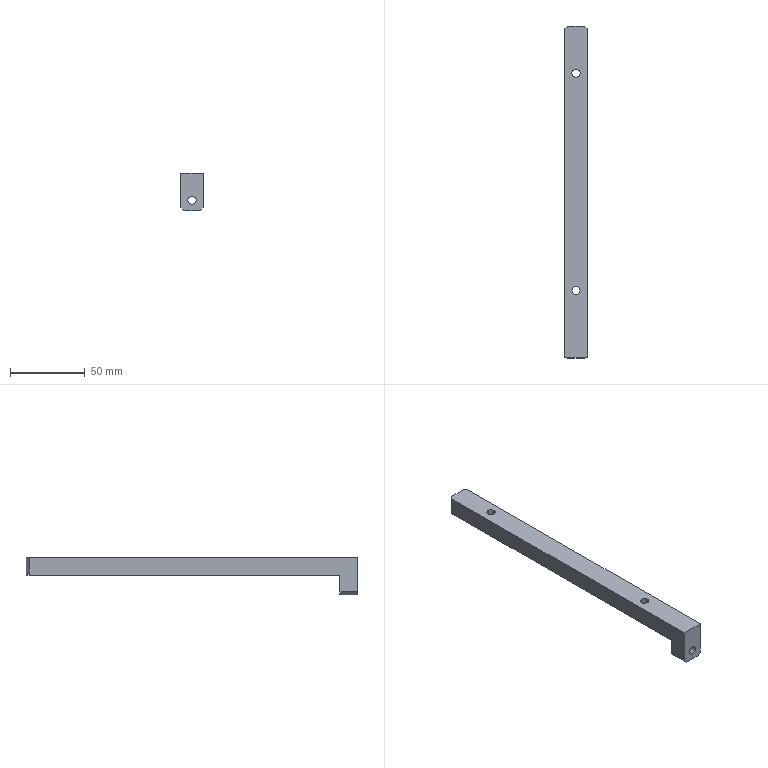Part | SolidWorks | features HoleWzd 2, Chamfer 1, Extrusion 1 | 1 solid | 24 faces | box 15 x 221.5 x 25 mm | volume 40634 mm3 | plane 14 | cylinder 10 | commonest cylinder face diameters 5.5 x6 10 x4
STEP:
#1=CARTESIAN_POINT('',(7.5,12.,-15.25));
#2=VERTEX_POINT('',#1);
#3=CARTESIAN_POINT('',(7.5,12.,-20.75));
#4=VERTEX_POINT('',#3);
#5=CARTESIAN_POINT('',(7.5,12.,-18.));
#6=DIRECTION('',(0.,-1.,0.));
#7=DIRECTION('',(0.,0.,-1.));
#8=AXIS2_PLACEMENT_3D('',#5,#6,#7);
#9=CIRCLE('',#8,2.75);
#10=EDGE_CURVE('',#2,#4,#9,.T.);
#11=ORIENTED_EDGE('',*,*,#10,.F.);
#12=CARTESIAN_POINT('',(7.5,0.,-15.25));
#13=VERTEX_POINT('',#12);
#14=CARTESIAN_POINT('',(7.5,0.,-15.25));
#15=DIRECTION('',(0.,-1.,0.));
#16=VECTOR('',#15,1000.);
#17=LINE('',#14,#16);
#18=EDGE_CURVE('',#2,#13,#17,.T.);
#19=ORIENTED_EDGE('',*,*,#18,.T.);
#20=CARTESIAN_POINT('',(7.5,0.,-20.75));
#21=VERTEX_POINT('',#20);
#22=CARTESIAN_POINT('',(7.5,0.,-18.));
#23=DIRECTION('',(0.,-1.,0.));
#24=DIRECTION('',(0.,0.,-1.));
#25=AXIS2_PLACEMENT_3D('',#22,#23,#24);
#26=CIRCLE('',#25,2.75);
#27=EDGE_CURVE('',#13,#21,#26,.T.);
#28=ORIENTED_EDGE('',*,*,#27,.T.);
#29=CARTESIAN_POINT('',(7.5,0.,-20.75));
#30=DIRECTION('',(0.,-1.,0.));
#31=VECTOR('',#30,1000.);
#32=LINE('',#29,#31);
#33=EDGE_CURVE('',#4,#21,#32,.T.);
#34=ORIENTED_EDGE('',*,*,#33,.F.);
#35=EDGE_LOOP('',(#11,#19,#28,#34));
#36=FACE_OUTER_BOUND('',#35,.T.);
#37=CARTESIAN_POINT('',(7.5,0.,-18.));
#38=DIRECTION('',(0.,-1.,0.));
#39=DIRECTION('',(0.,0.,-1.));
#40=AXIS2_PLACEMENT_3D('',#37,#38,#39);
#41=CYLINDRICAL_SURFACE('',#40,2.75);
#42=ADVANCED_FACE('',(#36),#41,.F.);
#43=CARTESIAN_POINT('',(7.5,185.,-6.3));
#44=VERTEX_POINT('',#43);
#45=CARTESIAN_POINT('',(7.5,195.,-6.3));
#46=VERTEX_POINT('',#45);
#47=CARTESIAN_POINT('',(7.5,190.,-6.3));
#48=DIRECTION('',(0.,0.,-1.));
#49=DIRECTION('',(0.,1.,0.));
#50=AXIS2_PLACEMENT_3D('',#47,#48,#49);
#51=CIRCLE('',#50,5.);
#52=EDGE_CURVE('',#44,#46,#51,.T.);
#53=ORIENTED_EDGE('',*,*,#52,.F.);
#54=CARTESIAN_POINT('',(7.5,185.,-12.));
#55=VERTEX_POINT('',#54);
#56=CARTESIAN_POINT('',(7.5,185.,-12.));
#57=DIRECTION('',(0.,0.,-1.));
#58=VECTOR('',#57,1000.);
#59=LINE('',#56,#58);
#60=EDGE_CURVE('',#44,#55,#59,.T.);
#61=ORIENTED_EDGE('',*,*,#60,.T.);
#62=CARTESIAN_POINT('',(7.5,195.,-12.));
#63=VERTEX_POINT('',#62);
#64=CARTESIAN_POINT('',(7.5,190.,-12.));
#65=DIRECTION('',(0.,0.,-1.));
#66=DIRECTION('',(0.,1.,0.));
#67=AXIS2_PLACEMENT_3D('',#64,#65,#66);
#68=CIRCLE('',#67,5.);
#69=EDGE_CURVE('',#55,#63,#68,.T.);
#70=ORIENTED_EDGE('',*,*,#69,.T.);
#71=CARTESIAN_POINT('',(7.5,195.,-12.));
#72=DIRECTION('',(0.,0.,-1.));
#73=VECTOR('',#72,1000.);
#74=LINE('',#71,#73);
#75=EDGE_CURVE('',#46,#63,#74,.T.);
#76=ORIENTED_EDGE('',*,*,#75,.F.);
#77=EDGE_LOOP('',(#53,#61,#70,#76));
#78=FACE_OUTER_BOUND('',#77,.T.);
#79=CARTESIAN_POINT('',(7.5,190.,-12.));
#80=DIRECTION('',(0.,0.,-1.));
#81=DIRECTION('',(0.,1.,0.));
#82=AXIS2_PLACEMENT_3D('',#79,#80,#81);
#83=CYLINDRICAL_SURFACE('',#82,5.);
#84=ADVANCED_FACE('',(#78),#83,.F.);
#85=CARTESIAN_POINT('',(7.5,187.25,0.));
#86=VERTEX_POINT('',#85);
#87=CARTESIAN_POINT('',(7.5,192.75,0.));
#88=VERTEX_POINT('',#87);
#89=CARTESIAN_POINT('',(7.5,190.,0.));
#90=DIRECTION('',(0.,0.,-1.));
#91=DIRECTION('',(0.,1.,0.));
#92=AXIS2_PLACEMENT_3D('',#89,#90,#91);
#93=CIRCLE('',#92,2.75);
#94=EDGE_CURVE('',#86,#88,#93,.T.);
#95=ORIENTED_EDGE('',*,*,#94,.F.);
#96=CARTESIAN_POINT('',(7.5,187.25,-6.3));
#97=VERTEX_POINT('',#96);
#98=CARTESIAN_POINT('',(7.5,187.25,-12.));
#99=DIRECTION('',(0.,0.,-1.));
#100=VECTOR('',#99,1000.);
#101=LINE('',#98,#100);
#102=EDGE_CURVE('',#86,#97,#101,.T.);
#103=ORIENTED_EDGE('',*,*,#102,.T.);
#104=CARTESIAN_POINT('',(7.5,192.75,-6.3));
#105=VERTEX_POINT('',#104);
#106=CARTESIAN_POINT('',(7.5,190.,-6.3));
#107=DIRECTION('',(0.,0.,-1.));
#108=DIRECTION('',(0.,1.,0.));
#109=AXIS2_PLACEMENT_3D('',#106,#107,#108);
#110=CIRCLE('',#109,2.75);
#111=EDGE_CURVE('',#97,#105,#110,.T.);
#112=ORIENTED_EDGE('',*,*,#111,.T.);
#113=CARTESIAN_POINT('',(7.5,192.75,-12.));
#114=DIRECTION('',(0.,0.,-1.));
#115=VECTOR('',#114,1000.);
#116=LINE('',#113,#115);
#117=EDGE_CURVE('',#88,#105,#116,.T.);
#118=ORIENTED_EDGE('',*,*,#117,.F.);
#119=EDGE_LOOP('',(#95,#103,#112,#118));
#120=FACE_OUTER_BOUND('',#119,.T.);
#121=CARTESIAN_POINT('',(7.5,190.,-12.));
#122=DIRECTION('',(0.,0.,-1.));
#123=DIRECTION('',(0.,1.,0.));
#124=AXIS2_PLACEMENT_3D('',#121,#122,#123);
#125=CYLINDRICAL_SURFACE('',#124,2.75);
#126=ADVANCED_FACE('',(#120),#125,.F.);
#127=CARTESIAN_POINT('',(7.5,40.,-6.3));
#128=VERTEX_POINT('',#127);
#129=CARTESIAN_POINT('',(7.5,50.,-6.3));
#130=VERTEX_POINT('',#129);
#131=CARTESIAN_POINT('',(7.5,45.,-6.3));
#132=DIRECTION('',(0.,0.,-1.));
#133=DIRECTION('',(0.,1.,0.));
#134=AXIS2_PLACEMENT_3D('',#131,#132,#133);
#135=CIRCLE('',#134,5.);
#136=EDGE_CURVE('',#128,#130,#135,.T.);
#137=ORIENTED_EDGE('',*,*,#136,.F.);
#138=CARTESIAN_POINT('',(7.5,40.,-12.));
#139=VERTEX_POINT('',#138);
#140=CARTESIAN_POINT('',(7.5,40.,-12.));
#141=DIRECTION('',(0.,0.,-1.));
#142=VECTOR('',#141,1000.);
#143=LINE('',#140,#142);
#144=EDGE_CURVE('',#128,#139,#143,.T.);
#145=ORIENTED_EDGE('',*,*,#144,.T.);
#146=CARTESIAN_POINT('',(7.5,50.,-12.));
#147=VERTEX_POINT('',#146);
#148=CARTESIAN_POINT('',(7.5,45.,-12.));
#149=DIRECTION('',(0.,0.,-1.));
#150=DIRECTION('',(0.,1.,0.));
#151=AXIS2_PLACEMENT_3D('',#148,#149,#150);
#152=CIRCLE('',#151,5.);
#153=EDGE_CURVE('',#139,#147,#152,.T.);
#154=ORIENTED_EDGE('',*,*,#153,.T.);
#155=CARTESIAN_POINT('',(7.5,50.,-12.));
#156=DIRECTION('',(0.,0.,-1.));
#157=VECTOR('',#156,1000.);
#158=LINE('',#155,#157);
#159=EDGE_CURVE('',#130,#147,#158,.T.);
#160=ORIENTED_EDGE('',*,*,#159,.F.);
#161=EDGE_LOOP('',(#137,#145,#154,#160));
#162=FACE_OUTER_BOUND('',#161,.T.);
#163=CARTESIAN_POINT('',(7.5,45.,-12.));
#164=DIRECTION('',(0.,0.,-1.));
#165=DIRECTION('',(0.,1.,0.));
#166=AXIS2_PLACEMENT_3D('',#163,#164,#165);
#167=CYLINDRICAL_SURFACE('',#166,5.);
#168=ADVANCED_FACE('',(#162),#167,.F.);
#169=CARTESIAN_POINT('',(7.5,42.25,0.));
#170=VERTEX_POINT('',#169);
#171=CARTESIAN_POINT('',(7.5,47.75,0.));
#172=VERTEX_POINT('',#171);
#173=CARTESIAN_POINT('',(7.5,45.,0.));
#174=DIRECTION('',(0.,0.,-1.));
#175=DIRECTION('',(0.,1.,0.));
#176=AXIS2_PLACEMENT_3D('',#173,#174,#175);
#177=CIRCLE('',#176,2.75);
#178=EDGE_CURVE('',#170,#172,#177,.T.);
#179=ORIENTED_EDGE('',*,*,#178,.F.);
#180=CARTESIAN_POINT('',(7.5,42.25,-6.3));
#181=VERTEX_POINT('',#180);
#182=CARTESIAN_POINT('',(7.5,42.25,-12.));
#183=DIRECTION('',(0.,0.,-1.));
#184=VECTOR('',#183,1000.);
#185=LINE('',#182,#184);
#186=EDGE_CURVE('',#170,#181,#185,.T.);
#187=ORIENTED_EDGE('',*,*,#186,.T.);
#188=CARTESIAN_POINT('',(7.5,47.75,-6.3));
#189=VERTEX_POINT('',#188);
#190=CARTESIAN_POINT('',(7.5,45.,-6.3));
#191=DIRECTION('',(0.,0.,-1.));
#192=DIRECTION('',(0.,1.,0.));
#193=AXIS2_PLACEMENT_3D('',#190,#191,#192);
#194=CIRCLE('',#193,2.75);
#195=EDGE_CURVE('',#181,#189,#194,.T.);
#196=ORIENTED_EDGE('',*,*,#195,.T.);
#197=CARTESIAN_POINT('',(7.5,47.75,-12.));
#198=DIRECTION('',(0.,0.,-1.));
#199=VECTOR('',#198,1000.);
#200=LINE('',#197,#199);
#201=EDGE_CURVE('',#172,#189,#200,.T.);
#202=ORIENTED_EDGE('',*,*,#201,.F.);
#203=EDGE_LOOP('',(#179,#187,#196,#202));
#204=FACE_OUTER_BOUND('',#203,.T.);
#205=CARTESIAN_POINT('',(7.5,45.,-12.));
#206=DIRECTION('',(0.,0.,-1.));
#207=DIRECTION('',(0.,1.,0.));
#208=AXIS2_PLACEMENT_3D('',#205,#206,#207);
#209=CYLINDRICAL_SURFACE('',#208,2.75);
#210=ADVANCED_FACE('',(#204),#209,.F.);
#211=CARTESIAN_POINT('',(7.5,190.,0.));
#212=DIRECTION('',(0.,0.,-1.));
#213=DIRECTION('',(0.,1.,0.));
#214=AXIS2_PLACEMENT_3D('',#211,#212,#213);
#215=CIRCLE('',#214,2.75);
#216=EDGE_CURVE('',#88,#86,#215,.T.);
#217=ORIENTED_EDGE('',*,*,#216,.T.);
#218=ORIENTED_EDGE('',*,*,#94,.T.);
#219=EDGE_LOOP('',(#217,#218));
#220=FACE_BOUND('',#219,.T.);
#221=CARTESIAN_POINT('',(7.5,45.,0.));
#222=DIRECTION('',(0.,0.,-1.));
#223=DIRECTION('',(0.,1.,0.));
#224=AXIS2_PLACEMENT_3D('',#221,#222,#223);
#225=CIRCLE('',#224,2.75);
#226=EDGE_CURVE('',#172,#170,#225,.T.);
#227=ORIENTED_EDGE('',*,*,#226,.T.);
#228=ORIENTED_EDGE('',*,*,#178,.T.);
#229=EDGE_LOOP('',(#227,#228));
#230=FACE_BOUND('',#229,.T.);
#231=CARTESIAN_POINT('',(13.,221.5,0.));
#232=VERTEX_POINT('',#231);
#233=CARTESIAN_POINT('',(2.,221.5,0.));
#234=VERTEX_POINT('',#233);
#235=CARTESIAN_POINT('',(15.,221.5,0.));
#236=DIRECTION('',(-1.,0.,0.));
#237=VECTOR('',#236,1000.);
#238=LINE('',#235,#237);
#239=EDGE_CURVE('',#232,#234,#238,.T.);
#240=ORIENTED_EDGE('',*,*,#239,.T.);
#241=CARTESIAN_POINT('',(0.,219.5,0.));
#242=VERTEX_POINT('',#241);
#243=CARTESIAN_POINT('',(2.,221.5,0.));
#244=DIRECTION('',(-0.7071,-0.7071,0.));
#245=VECTOR('',#244,1000.);
#246=LINE('',#243,#245);
#247=EDGE_CURVE('',#234,#242,#246,.T.);
#248=ORIENTED_EDGE('',*,*,#247,.T.);
#249=CARTESIAN_POINT('',(0.,0.,0.));
#250=VERTEX_POINT('',#249);
#251=CARTESIAN_POINT('',(0.,221.5,0.));
#252=DIRECTION('',(0.,-1.,0.));
#253=VECTOR('',#252,1000.);
#254=LINE('',#251,#253);
#255=EDGE_CURVE('',#242,#250,#254,.T.);
#256=ORIENTED_EDGE('',*,*,#255,.T.);
#257=CARTESIAN_POINT('',(15.,0.,0.));
#258=VERTEX_POINT('',#257);
#259=CARTESIAN_POINT('',(15.,0.,0.));
#260=DIRECTION('',(-1.,0.,0.));
#261=VECTOR('',#260,1000.);
#262=LINE('',#259,#261);
#263=EDGE_CURVE('',#258,#250,#262,.T.);
#264=ORIENTED_EDGE('',*,*,#263,.F.);
#265=CARTESIAN_POINT('',(15.,219.5,0.));
#266=VERTEX_POINT('',#265);
#267=CARTESIAN_POINT('',(15.,221.5,0.));
#268=DIRECTION('',(0.,-1.,0.));
#269=VECTOR('',#268,1000.);
#270=LINE('',#267,#269);
#271=EDGE_CURVE('',#266,#258,#270,.T.);
#272=ORIENTED_EDGE('',*,*,#271,.F.);
#273=CARTESIAN_POINT('',(15.,219.5,0.));
#274=DIRECTION('',(-0.7071,0.7071,0.));
#275=VECTOR('',#274,1000.);
#276=LINE('',#273,#275);
#277=EDGE_CURVE('',#266,#232,#276,.T.);
#278=ORIENTED_EDGE('',*,*,#277,.T.);
#279=EDGE_LOOP('',(#240,#248,#256,#264,#272,#278));
#280=FACE_OUTER_BOUND('',#279,.T.);
#281=CARTESIAN_POINT('',(15.,221.5,0.));
#282=DIRECTION('',(0.,0.,-1.));
#283=DIRECTION('',(-1.,0.,0.));
#284=AXIS2_PLACEMENT_3D('',#281,#282,#283);
#285=PLANE('',#284);
#286=ADVANCED_FACE('',(#220,#230,#280),#285,.F.);
#287=CARTESIAN_POINT('',(7.5,0.,-18.));
#288=DIRECTION('',(0.,-1.,0.));
#289=DIRECTION('',(0.,0.,-1.));
#290=AXIS2_PLACEMENT_3D('',#287,#288,#289);
#291=CIRCLE('',#290,2.75);
#292=EDGE_CURVE('',#21,#13,#291,.T.);
#293=ORIENTED_EDGE('',*,*,#292,.F.);
#294=ORIENTED_EDGE('',*,*,#27,.F.);
#295=EDGE_LOOP('',(#293,#294));
#296=FACE_BOUND('',#295,.T.);
#297=CARTESIAN_POINT('',(0.,0.,-23.));
#298=VERTEX_POINT('',#297);
#299=CARTESIAN_POINT('',(0.,0.,0.));
#300=DIRECTION('',(0.,0.,-1.));
#301=VECTOR('',#300,1000.);
#302=LINE('',#299,#301);
#303=EDGE_CURVE('',#250,#298,#302,.T.);
#304=ORIENTED_EDGE('',*,*,#303,.T.);
#305=CARTESIAN_POINT('',(2.,0.,-25.));
#306=VERTEX_POINT('',#305);
#307=CARTESIAN_POINT('',(2.,0.,-25.));
#308=DIRECTION('',(0.7071,0.,-0.7071));
#309=VECTOR('',#308,1000.);
#310=LINE('',#307,#309);
#311=EDGE_CURVE('',#298,#306,#310,.T.);
#312=ORIENTED_EDGE('',*,*,#311,.T.);
#313=CARTESIAN_POINT('',(13.,0.,-25.));
#314=VERTEX_POINT('',#313);
#315=CARTESIAN_POINT('',(15.,0.,-25.));
#316=DIRECTION('',(-1.,0.,0.));
#317=VECTOR('',#316,1000.);
#318=LINE('',#315,#317);
#319=EDGE_CURVE('',#314,#306,#318,.T.);
#320=ORIENTED_EDGE('',*,*,#319,.F.);
#321=CARTESIAN_POINT('',(15.,0.,-23.));
#322=VERTEX_POINT('',#321);
#323=CARTESIAN_POINT('',(15.,0.,-23.));
#324=DIRECTION('',(0.7071,0.,0.7071));
#325=VECTOR('',#324,1000.);
#326=LINE('',#323,#325);
#327=EDGE_CURVE('',#314,#322,#326,.T.);
#328=ORIENTED_EDGE('',*,*,#327,.T.);
#329=CARTESIAN_POINT('',(15.,0.,0.));
#330=DIRECTION('',(0.,0.,-1.));
#331=VECTOR('',#330,1000.);
#332=LINE('',#329,#331);
#333=EDGE_CURVE('',#258,#322,#332,.T.);
#334=ORIENTED_EDGE('',*,*,#333,.F.);
#335=ORIENTED_EDGE('',*,*,#263,.T.);
#336=EDGE_LOOP('',(#304,#312,#320,#328,#334,#335));
#337=FACE_OUTER_BOUND('',#336,.T.);
#338=CARTESIAN_POINT('',(15.,0.,0.));
#339=DIRECTION('',(0.,1.,0.));
#340=DIRECTION('',(0.,0.,1.));
#341=AXIS2_PLACEMENT_3D('',#338,#339,#340);
#342=PLANE('',#341);
#343=ADVANCED_FACE('',(#296,#337),#342,.F.);
#344=ORIENTED_EDGE('',*,*,#319,.T.);
#345=CARTESIAN_POINT('',(2.,12.,-25.));
#346=VERTEX_POINT('',#345);
#347=CARTESIAN_POINT('',(2.,0.,-25.));
#348=DIRECTION('',(0.,1.,0.));
#349=VECTOR('',#348,1000.);
#350=LINE('',#347,#349);
#351=EDGE_CURVE('',#306,#346,#350,.T.);
#352=ORIENTED_EDGE('',*,*,#351,.T.);
#353=CARTESIAN_POINT('',(13.,12.,-25.));
#354=VERTEX_POINT('',#353);
#355=CARTESIAN_POINT('',(15.,12.,-25.));
#356=DIRECTION('',(-1.,0.,0.));
#357=VECTOR('',#356,1000.);
#358=LINE('',#355,#357);
#359=EDGE_CURVE('',#354,#346,#358,.T.);
#360=ORIENTED_EDGE('',*,*,#359,.F.);
#361=CARTESIAN_POINT('',(13.,0.,-25.));
#362=DIRECTION('',(0.,-1.,0.));
#363=VECTOR('',#362,1000.);
#364=LINE('',#361,#363);
#365=EDGE_CURVE('',#354,#314,#364,.T.);
#366=ORIENTED_EDGE('',*,*,#365,.T.);
#367=EDGE_LOOP('',(#344,#352,#360,#366));
#368=FACE_OUTER_BOUND('',#367,.T.);
#369=CARTESIAN_POINT('',(15.,0.,-25.));
#370=DIRECTION('',(0.,0.,1.));
#371=DIRECTION('',(1.,0.,0.));
#372=AXIS2_PLACEMENT_3D('',#369,#370,#371);
#373=PLANE('',#372);
#374=ADVANCED_FACE('',(#368),#373,.F.);
#375=CARTESIAN_POINT('',(7.5,12.,-18.));
#376=DIRECTION('',(0.,-1.,0.));
#377=DIRECTION('',(0.,0.,-1.));
#378=AXIS2_PLACEMENT_3D('',#375,#376,#377);
#379=CIRCLE('',#378,2.75);
#380=EDGE_CURVE('',#4,#2,#379,.T.);
#381=ORIENTED_EDGE('',*,*,#380,.T.);
#382=ORIENTED_EDGE('',*,*,#10,.T.);
#383=EDGE_LOOP('',(#381,#382));
#384=FACE_BOUND('',#383,.T.);
#385=ORIENTED_EDGE('',*,*,#359,.T.);
#386=CARTESIAN_POINT('',(0.,12.,-23.));
#387=VERTEX_POINT('',#386);
#388=CARTESIAN_POINT('',(2.,12.,-25.));
#389=DIRECTION('',(-0.7071,0.,0.7071));
#390=VECTOR('',#389,1000.);
#391=LINE('',#388,#390);
#392=EDGE_CURVE('',#346,#387,#391,.T.);
#393=ORIENTED_EDGE('',*,*,#392,.T.);
#394=CARTESIAN_POINT('',(0.,12.,-12.));
#395=VERTEX_POINT('',#394);
#396=CARTESIAN_POINT('',(0.,12.,-25.));
#397=DIRECTION('',(0.,0.,1.));
#398=VECTOR('',#397,1000.);
#399=LINE('',#396,#398);
#400=EDGE_CURVE('',#387,#395,#399,.T.);
#401=ORIENTED_EDGE('',*,*,#400,.T.);
#402=CARTESIAN_POINT('',(15.,12.,-12.));
#403=VERTEX_POINT('',#402);
#404=CARTESIAN_POINT('',(15.,12.,-12.));
#405=DIRECTION('',(-1.,0.,0.));
#406=VECTOR('',#405,1000.);
#407=LINE('',#404,#406);
#408=EDGE_CURVE('',#403,#395,#407,.T.);
#409=ORIENTED_EDGE('',*,*,#408,.F.);
#410=CARTESIAN_POINT('',(15.,12.,-23.));
#411=VERTEX_POINT('',#410);
#412=CARTESIAN_POINT('',(15.,12.,-25.));
#413=DIRECTION('',(0.,0.,1.));
#414=VECTOR('',#413,1000.);
#415=LINE('',#412,#414);
#416=EDGE_CURVE('',#411,#403,#415,.T.);
#417=ORIENTED_EDGE('',*,*,#416,.F.);
#418=CARTESIAN_POINT('',(15.,12.,-23.));
#419=DIRECTION('',(-0.7071,0.,-0.7071));
#420=VECTOR('',#419,1000.);
#421=LINE('',#418,#420);
#422=EDGE_CURVE('',#411,#354,#421,.T.);
#423=ORIENTED_EDGE('',*,*,#422,.T.);
#424=EDGE_LOOP('',(#385,#393,#401,#409,#417,#423));
#425=FACE_OUTER_BOUND('',#424,.T.);
#426=CARTESIAN_POINT('',(15.,12.,-25.));
#427=DIRECTION('',(0.,-1.,0.));
#428=DIRECTION('',(0.,0.,-1.));
#429=AXIS2_PLACEMENT_3D('',#426,#427,#428);
#430=PLANE('',#429);
#431=ADVANCED_FACE('',(#384,#425),#430,.F.);
#432=CARTESIAN_POINT('',(7.5,190.,-12.));
#433=DIRECTION('',(0.,0.,-1.));
#434=DIRECTION('',(0.,1.,0.));
#435=AXIS2_PLACEMENT_3D('',#432,#433,#434);
#436=CIRCLE('',#435,5.);
#437=EDGE_CURVE('',#63,#55,#436,.T.);
#438=ORIENTED_EDGE('',*,*,#437,.F.);
#439=ORIENTED_EDGE('',*,*,#69,.F.);
#440=EDGE_LOOP('',(#438,#439));
#441=FACE_BOUND('',#440,.T.);
#442=CARTESIAN_POINT('',(7.5,45.,-12.));
#443=DIRECTION('',(0.,0.,-1.));
#444=DIRECTION('',(0.,1.,0.));
#445=AXIS2_PLACEMENT_3D('',#442,#443,#444);
#446=CIRCLE('',#445,5.);
#447=EDGE_CURVE('',#147,#139,#446,.T.);
#448=ORIENTED_EDGE('',*,*,#447,.F.);
#449=ORIENTED_EDGE('',*,*,#153,.F.);
#450=EDGE_LOOP('',(#448,#449));
#451=FACE_BOUND('',#450,.T.);
#452=CARTESIAN_POINT('',(0.,219.5,-12.));
#453=VERTEX_POINT('',#452);
#454=CARTESIAN_POINT('',(0.,12.,-12.));
#455=DIRECTION('',(0.,1.,0.));
#456=VECTOR('',#455,1000.);
#457=LINE('',#454,#456);
#458=EDGE_CURVE('',#395,#453,#457,.T.);
#459=ORIENTED_EDGE('',*,*,#458,.T.);
#460=CARTESIAN_POINT('',(2.,221.5,-12.));
#461=VERTEX_POINT('',#460);
#462=CARTESIAN_POINT('',(2.,221.5,-12.));
#463=DIRECTION('',(0.7071,0.7071,0.));
#464=VECTOR('',#463,1000.);
#465=LINE('',#462,#464);
#466=EDGE_CURVE('',#453,#461,#465,.T.);
#467=ORIENTED_EDGE('',*,*,#466,.T.);
#468=CARTESIAN_POINT('',(13.,221.5,-12.));
#469=VERTEX_POINT('',#468);
#470=CARTESIAN_POINT('',(15.,221.5,-12.));
#471=DIRECTION('',(-1.,0.,0.));
#472=VECTOR('',#471,1000.);
#473=LINE('',#470,#472);
#474=EDGE_CURVE('',#469,#461,#473,.T.);
#475=ORIENTED_EDGE('',*,*,#474,.F.);
#476=CARTESIAN_POINT('',(15.,219.5,-12.));
#477=VERTEX_POINT('',#476);
#478=CARTESIAN_POINT('',(15.,219.5,-12.));
#479=DIRECTION('',(0.7071,-0.7071,0.));
#480=VECTOR('',#479,1000.);
#481=LINE('',#478,#480);
#482=EDGE_CURVE('',#469,#477,#481,.T.);
#483=ORIENTED_EDGE('',*,*,#482,.T.);
#484=CARTESIAN_POINT('',(15.,12.,-12.));
#485=DIRECTION('',(0.,1.,0.));
#486=VECTOR('',#485,1000.);
#487=LINE('',#484,#486);
#488=EDGE_CURVE('',#403,#477,#487,.T.);
#489=ORIENTED_EDGE('',*,*,#488,.F.);
#490=ORIENTED_EDGE('',*,*,#408,.T.);
#491=EDGE_LOOP('',(#459,#467,#475,#483,#489,#490));
#492=FACE_OUTER_BOUND('',#491,.T.);
#493=CARTESIAN_POINT('',(15.,12.,-12.));
#494=DIRECTION('',(0.,0.,1.));
#495=DIRECTION('',(0.,-1.,0.));
#496=AXIS2_PLACEMENT_3D('',#493,#494,#495);
#497=PLANE('',#496);
#498=ADVANCED_FACE('',(#441,#451,#492),#497,.F.);
#499=ORIENTED_EDGE('',*,*,#474,.T.);
#500=CARTESIAN_POINT('',(2.,221.5,-12.));
#501=DIRECTION('',(0.,0.,1.));
#502=VECTOR('',#501,1000.);
#503=LINE('',#500,#502);
#504=EDGE_CURVE('',#461,#234,#503,.T.);
#505=ORIENTED_EDGE('',*,*,#504,.T.);
#506=ORIENTED_EDGE('',*,*,#239,.F.);
#507=CARTESIAN_POINT('',(13.,221.5,-12.));
#508=DIRECTION('',(0.,0.,-1.));
#509=VECTOR('',#508,1000.);
#510=LINE('',#507,#509);
#511=EDGE_CURVE('',#232,#469,#510,.T.);
#512=ORIENTED_EDGE('',*,*,#511,.T.);
#513=EDGE_LOOP('',(#499,#505,#506,#512));
#514=FACE_OUTER_BOUND('',#513,.T.);
#515=CARTESIAN_POINT('',(15.,221.5,-12.));
#516=DIRECTION('',(0.,-1.,0.));
#517=DIRECTION('',(0.,0.,-1.));
#518=AXIS2_PLACEMENT_3D('',#515,#516,#517);
#519=PLANE('',#518);
#520=ADVANCED_FACE('',(#514),#519,.F.);
#521=ORIENTED_EDGE('',*,*,#333,.T.);
#522=CARTESIAN_POINT('',(15.,12.,-23.));
#523=DIRECTION('',(0.,1.,0.));
#524=VECTOR('',#523,1000.);
#525=LINE('',#522,#524);
#526=EDGE_CURVE('',#322,#411,#525,.T.);
#527=ORIENTED_EDGE('',*,*,#526,.T.);
#528=ORIENTED_EDGE('',*,*,#416,.T.);
#529=ORIENTED_EDGE('',*,*,#488,.T.);
#530=CARTESIAN_POINT('',(15.,219.5,0.));
#531=DIRECTION('',(0.,0.,1.));
#532=VECTOR('',#531,1000.);
#533=LINE('',#530,#532);
#534=EDGE_CURVE('',#477,#266,#533,.T.);
#535=ORIENTED_EDGE('',*,*,#534,.T.);
#536=ORIENTED_EDGE('',*,*,#271,.T.);
#537=EDGE_LOOP('',(#521,#527,#528,#529,#535,#536));
#538=FACE_OUTER_BOUND('',#537,.T.);
#539=CARTESIAN_POINT('',(15.,0.,0.));
#540=DIRECTION('',(1.,0.,0.));
#541=DIRECTION('',(0.,0.,-1.));
#542=AXIS2_PLACEMENT_3D('',#539,#540,#541);
#543=PLANE('',#542);
#544=ADVANCED_FACE('',(#538),#543,.T.);
#545=ORIENTED_EDGE('',*,*,#400,.F.);
#546=CARTESIAN_POINT('',(0.,0.,-23.));
#547=DIRECTION('',(0.,-1.,0.));
#548=VECTOR('',#547,1000.);
#549=LINE('',#546,#548);
#550=EDGE_CURVE('',#387,#298,#549,.T.);
#551=ORIENTED_EDGE('',*,*,#550,.T.);
#552=ORIENTED_EDGE('',*,*,#303,.F.);
#553=ORIENTED_EDGE('',*,*,#255,.F.);
#554=CARTESIAN_POINT('',(0.,219.5,0.));
#555=DIRECTION('',(0.,0.,-1.));
#556=VECTOR('',#555,1000.);
#557=LINE('',#554,#556);
#558=EDGE_CURVE('',#242,#453,#557,.T.);
#559=ORIENTED_EDGE('',*,*,#558,.T.);
#560=ORIENTED_EDGE('',*,*,#458,.F.);
#561=EDGE_LOOP('',(#545,#551,#552,#553,#559,#560));
#562=FACE_OUTER_BOUND('',#561,.T.);
#563=CARTESIAN_POINT('',(0.,0.,0.));
#564=DIRECTION('',(1.,0.,0.));
#565=DIRECTION('',(0.,0.,-1.));
#566=AXIS2_PLACEMENT_3D('',#563,#564,#565);
#567=PLANE('',#566);
#568=ADVANCED_FACE('',(#562),#567,.F.);
#569=ORIENTED_EDGE('',*,*,#186,.F.);
#570=ORIENTED_EDGE('',*,*,#226,.F.);
#571=ORIENTED_EDGE('',*,*,#201,.T.);
#572=CARTESIAN_POINT('',(7.5,45.,-6.3));
#573=DIRECTION('',(0.,0.,-1.));
#574=DIRECTION('',(0.,1.,0.));
#575=AXIS2_PLACEMENT_3D('',#572,#573,#574);
#576=CIRCLE('',#575,2.75);
#577=EDGE_CURVE('',#189,#181,#576,.T.);
#578=ORIENTED_EDGE('',*,*,#577,.T.);
#579=EDGE_LOOP('',(#569,#570,#571,#578));
#580=FACE_OUTER_BOUND('',#579,.T.);
#581=CARTESIAN_POINT('',(7.5,45.,-12.));
#582=DIRECTION('',(0.,0.,-1.));
#583=DIRECTION('',(0.,1.,0.));
#584=AXIS2_PLACEMENT_3D('',#581,#582,#583);
#585=CYLINDRICAL_SURFACE('',#584,2.75);
#586=ADVANCED_FACE('',(#580),#585,.F.);
#587=ORIENTED_EDGE('',*,*,#577,.F.);
#588=ORIENTED_EDGE('',*,*,#195,.F.);
#589=EDGE_LOOP('',(#587,#588));
#590=FACE_BOUND('',#589,.T.);
#591=CARTESIAN_POINT('',(7.5,45.,-6.3));
#592=DIRECTION('',(0.,0.,-1.));
#593=DIRECTION('',(0.,1.,0.));
#594=AXIS2_PLACEMENT_3D('',#591,#592,#593);
#595=CIRCLE('',#594,5.);
#596=EDGE_CURVE('',#130,#128,#595,.T.);
#597=ORIENTED_EDGE('',*,*,#596,.T.);
#598=ORIENTED_EDGE('',*,*,#136,.T.);
#599=EDGE_LOOP('',(#597,#598));
#600=FACE_OUTER_BOUND('',#599,.T.);
#601=CARTESIAN_POINT('',(10.25,45.,-6.3));
#602=DIRECTION('',(0.,0.,1.));
#603=DIRECTION('',(0.,-1.,0.));
#604=AXIS2_PLACEMENT_3D('',#601,#602,#603);
#605=PLANE('',#604);
#606=ADVANCED_FACE('',(#590,#600),#605,.F.);
#607=ORIENTED_EDGE('',*,*,#144,.F.);
#608=ORIENTED_EDGE('',*,*,#596,.F.);
#609=ORIENTED_EDGE('',*,*,#159,.T.);
#610=ORIENTED_EDGE('',*,*,#447,.T.);
#611=EDGE_LOOP('',(#607,#608,#609,#610));
#612=FACE_OUTER_BOUND('',#611,.T.);
#613=CARTESIAN_POINT('',(7.5,45.,-12.));
#614=DIRECTION('',(0.,0.,-1.));
#615=DIRECTION('',(0.,1.,0.));
#616=AXIS2_PLACEMENT_3D('',#613,#614,#615);
#617=CYLINDRICAL_SURFACE('',#616,5.);
#618=ADVANCED_FACE('',(#612),#617,.F.);
#619=ORIENTED_EDGE('',*,*,#102,.F.);
#620=ORIENTED_EDGE('',*,*,#216,.F.);
#621=ORIENTED_EDGE('',*,*,#117,.T.);
#622=CARTESIAN_POINT('',(7.5,190.,-6.3));
#623=DIRECTION('',(0.,0.,-1.));
#624=DIRECTION('',(0.,1.,0.));
#625=AXIS2_PLACEMENT_3D('',#622,#623,#624);
#626=CIRCLE('',#625,2.75);
#627=EDGE_CURVE('',#105,#97,#626,.T.);
#628=ORIENTED_EDGE('',*,*,#627,.T.);
#629=EDGE_LOOP('',(#619,#620,#621,#628));
#630=FACE_OUTER_BOUND('',#629,.T.);
#631=CARTESIAN_POINT('',(7.5,190.,-12.));
#632=DIRECTION('',(0.,0.,-1.));
#633=DIRECTION('',(0.,1.,0.));
#634=AXIS2_PLACEMENT_3D('',#631,#632,#633);
#635=CYLINDRICAL_SURFACE('',#634,2.75);
#636=ADVANCED_FACE('',(#630),#635,.F.);
#637=ORIENTED_EDGE('',*,*,#627,.F.);
#638=ORIENTED_EDGE('',*,*,#111,.F.);
#639=EDGE_LOOP('',(#637,#638));
#640=FACE_BOUND('',#639,.T.);
#641=CARTESIAN_POINT('',(7.5,190.,-6.3));
#642=DIRECTION('',(0.,0.,-1.));
#643=DIRECTION('',(0.,1.,0.));
#644=AXIS2_PLACEMENT_3D('',#641,#642,#643);
#645=CIRCLE('',#644,5.);
#646=EDGE_CURVE('',#46,#44,#645,.T.);
#647=ORIENTED_EDGE('',*,*,#646,.T.);
#648=ORIENTED_EDGE('',*,*,#52,.T.);
#649=EDGE_LOOP('',(#647,#648));
#650=FACE_OUTER_BOUND('',#649,.T.);
#651=CARTESIAN_POINT('',(10.25,190.,-6.3));
#652=DIRECTION('',(0.,0.,1.));
#653=DIRECTION('',(0.,-1.,0.));
#654=AXIS2_PLACEMENT_3D('',#651,#652,#653);
#655=PLANE('',#654);
#656=ADVANCED_FACE('',(#640,#650),#655,.F.);
#657=ORIENTED_EDGE('',*,*,#60,.F.);
#658=ORIENTED_EDGE('',*,*,#646,.F.);
#659=ORIENTED_EDGE('',*,*,#75,.T.);
#660=ORIENTED_EDGE('',*,*,#437,.T.);
#661=EDGE_LOOP('',(#657,#658,#659,#660));
#662=FACE_OUTER_BOUND('',#661,.T.);
#663=CARTESIAN_POINT('',(7.5,190.,-12.));
#664=DIRECTION('',(0.,0.,-1.));
#665=DIRECTION('',(0.,1.,0.));
#666=AXIS2_PLACEMENT_3D('',#663,#664,#665);
#667=CYLINDRICAL_SURFACE('',#666,5.);
#668=ADVANCED_FACE('',(#662),#667,.F.);
#669=ORIENTED_EDGE('',*,*,#18,.F.);
#670=ORIENTED_EDGE('',*,*,#380,.F.);
#671=ORIENTED_EDGE('',*,*,#33,.T.);
#672=ORIENTED_EDGE('',*,*,#292,.T.);
#673=EDGE_LOOP('',(#669,#670,#671,#672));
#674=FACE_OUTER_BOUND('',#673,.T.);
#675=CARTESIAN_POINT('',(7.5,0.,-18.));
#676=DIRECTION('',(0.,-1.,0.));
#677=DIRECTION('',(0.,0.,-1.));
#678=AXIS2_PLACEMENT_3D('',#675,#676,#677);
#679=CYLINDRICAL_SURFACE('',#678,2.75);
#680=ADVANCED_FACE('',(#674),#679,.F.);
#681=ORIENTED_EDGE('',*,*,#311,.F.);
#682=ORIENTED_EDGE('',*,*,#550,.F.);
#683=ORIENTED_EDGE('',*,*,#392,.F.);
#684=ORIENTED_EDGE('',*,*,#351,.F.);
#685=EDGE_LOOP('',(#681,#682,#683,#684));
#686=FACE_OUTER_BOUND('',#685,.T.);
#687=CARTESIAN_POINT('',(2.,0.,-25.));
#688=DIRECTION('',(0.7071,0.,0.7071));
#689=DIRECTION('',(0.,1.,0.));
#690=AXIS2_PLACEMENT_3D('',#687,#688,#689);
#691=PLANE('',#690);
#692=ADVANCED_FACE('',(#686),#691,.F.);
#693=ORIENTED_EDGE('',*,*,#327,.F.);
#694=ORIENTED_EDGE('',*,*,#365,.F.);
#695=ORIENTED_EDGE('',*,*,#422,.F.);
#696=ORIENTED_EDGE('',*,*,#526,.F.);
#697=EDGE_LOOP('',(#693,#694,#695,#696));
#698=FACE_OUTER_BOUND('',#697,.T.);
#699=CARTESIAN_POINT('',(15.,0.,-23.));
#700=DIRECTION('',(0.7071,0.,-0.7071));
#701=DIRECTION('',(0.,-1.,0.));
#702=AXIS2_PLACEMENT_3D('',#699,#700,#701);
#703=PLANE('',#702);
#704=ADVANCED_FACE('',(#698),#703,.T.);
#705=ORIENTED_EDGE('',*,*,#466,.F.);
#706=ORIENTED_EDGE('',*,*,#558,.F.);
#707=ORIENTED_EDGE('',*,*,#247,.F.);
#708=ORIENTED_EDGE('',*,*,#504,.F.);
#709=EDGE_LOOP('',(#705,#706,#707,#708));
#710=FACE_OUTER_BOUND('',#709,.T.);
#711=CARTESIAN_POINT('',(2.,221.5,-12.));
#712=DIRECTION('',(0.7071,-0.7071,0.));
#713=DIRECTION('',(0.,0.,1.));
#714=AXIS2_PLACEMENT_3D('',#711,#712,#713);
#715=PLANE('',#714);
#716=ADVANCED_FACE('',(#710),#715,.F.);
#717=ORIENTED_EDGE('',*,*,#482,.F.);
#718=ORIENTED_EDGE('',*,*,#511,.F.);
#719=ORIENTED_EDGE('',*,*,#277,.F.);
#720=ORIENTED_EDGE('',*,*,#534,.F.);
#721=EDGE_LOOP('',(#717,#718,#719,#720));
#722=FACE_OUTER_BOUND('',#721,.T.);
#723=CARTESIAN_POINT('',(15.,219.5,0.));
#724=DIRECTION('',(0.7071,0.7071,0.));
#725=DIRECTION('',(0.,0.,-1.));
#726=AXIS2_PLACEMENT_3D('',#723,#724,#725);
#727=PLANE('',#726);
#728=ADVANCED_FACE('',(#722),#727,.T.);
#729=CLOSED_SHELL('',(#42,#84,#126,#168,#210,#286,#343,#374,#431,#498,#520,#544,#568,#586,#606,#618,#636,#656,#668,#680,#692,#704,#716,#728));
#730=MANIFOLD_SOLID_BREP('',#729);
#731=CARTESIAN_POINT('',(0.,0.,0.));
#732=DIRECTION('',(0.,0.,1.));
#733=DIRECTION('',(1.,0.,0.));
#734=AXIS2_PLACEMENT_3D('',#731,#732,#733);
#735=(LENGTH_UNIT()NAMED_UNIT(*)SI_UNIT(.MILLI.,.METRE.));
#736=UNCERTAINTY_MEASURE_WITH_UNIT(LENGTH_MEASURE(0.00001),#735,'','');
#737=(NAMED_UNIT(*)PLANE_ANGLE_UNIT()SI_UNIT($,.RADIAN.));
#738=(NAMED_UNIT(*)SI_UNIT($,.STERADIAN.)SOLID_ANGLE_UNIT());
#739=(GEOMETRIC_REPRESENTATION_CONTEXT(3)GLOBAL_UNCERTAINTY_ASSIGNED_CONTEXT((#736))GLOBAL_UNIT_ASSIGNED_CONTEXT((#735,#737,#738))REPRESENTATION_CONTEXT('',''));
#740=ADVANCED_BREP_SHAPE_REPRESENTATION('',(#730,#734),#739);